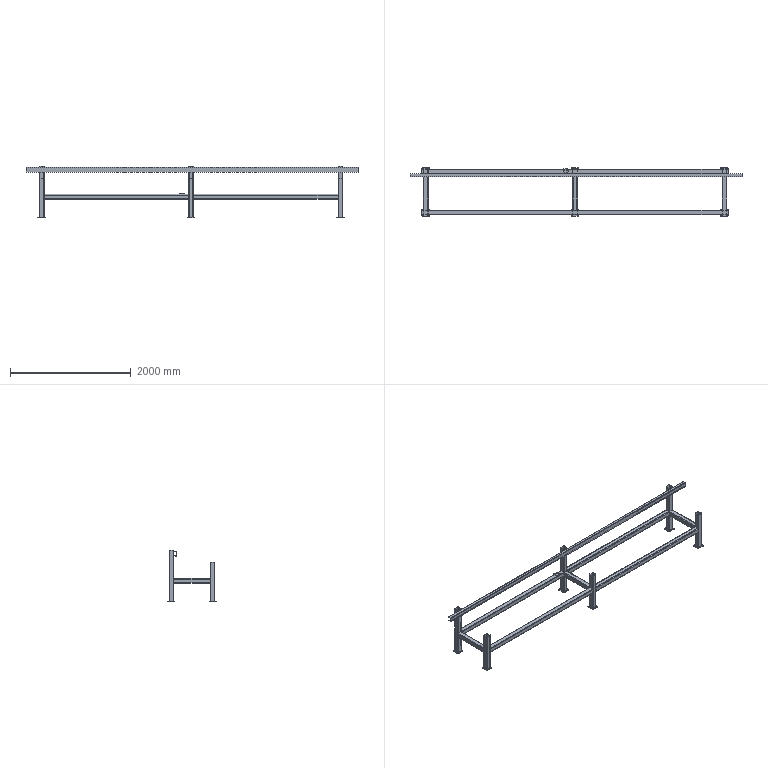Part | STEP file | 15 solids | 374 faces | box 5500 x 803.417 x 860 mm | volume 20632149 mm3 | cylinder 192 | plane 182 | commonest cylinder face diameters 14 x100 20 x76 4.2 x8 26.2 x4 8 x2 16 x2